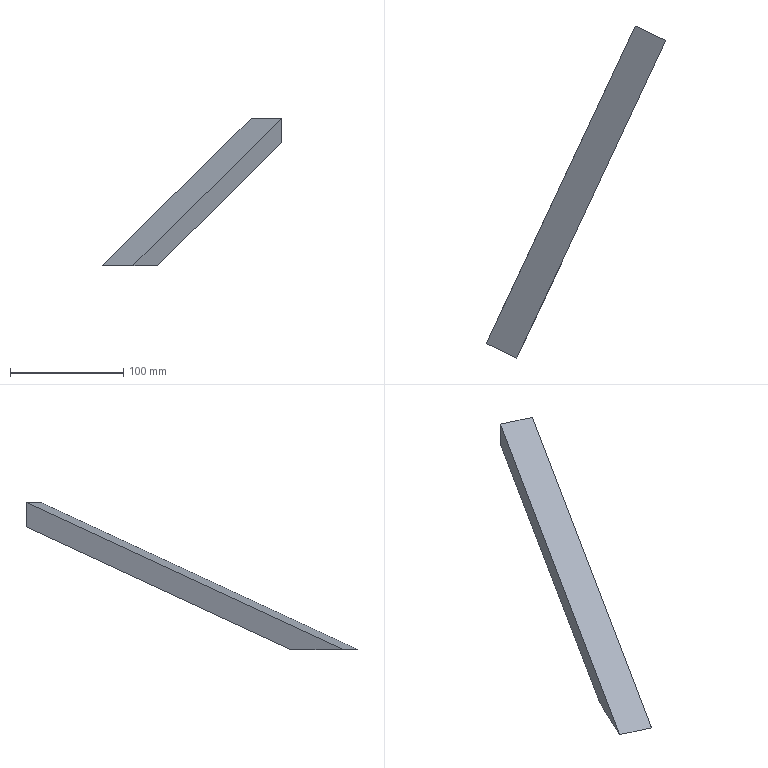Part | STEP file | Boss-Extrude 36 | 1 solid | 6 faces | box 158.76 x 293.326 x 130.156 mm | volume 184876 mm3 | plane 6
STEP:
#1=CARTESIAN_POINT('',(-1003.706,-516.863,2786.));
#2=VERTEX_POINT('',#1);
#3=CARTESIAN_POINT('',(-894.04,-283.039,2894.464));
#4=VERTEX_POINT('',#3);
#5=CARTESIAN_POINT('',(-894.04,-283.039,2894.464));
#6=DIRECTION('',(0.3915,0.8347,0.3872));
#7=VECTOR('',#6,1000.);
#8=LINE('',#5,#7);
#9=EDGE_CURVE('',#2,#4,#8,.T.);
#10=ORIENTED_EDGE('',*,*,#9,.F.);
#11=CARTESIAN_POINT('',(-1030.867,-504.124,2786.));
#12=VERTEX_POINT('',#11);
#13=CARTESIAN_POINT('',(-1030.867,-504.124,2786.));
#14=DIRECTION('',(0.9054,-0.4246,0.));
#15=VECTOR('',#14,1000.);
#16=LINE('',#13,#15);
#17=EDGE_CURVE('',#12,#2,#16,.T.);
#18=ORIENTED_EDGE('',*,*,#17,.F.);
#19=CARTESIAN_POINT('',(-921.201,-270.3,2894.464));
#20=VERTEX_POINT('',#19);
#21=CARTESIAN_POINT('',(-921.201,-270.3,2894.464));
#22=DIRECTION('',(0.3915,0.8347,0.3872));
#23=VECTOR('',#22,1000.);
#24=LINE('',#21,#23);
#25=EDGE_CURVE('',#12,#20,#24,.T.);
#26=ORIENTED_EDGE('',*,*,#25,.T.);
#27=CARTESIAN_POINT('',(-921.201,-270.3,2894.464));
#28=DIRECTION('',(0.9054,-0.4246,0.));
#29=VECTOR('',#28,1000.);
#30=LINE('',#27,#29);
#31=EDGE_CURVE('',#20,#4,#30,.T.);
#32=ORIENTED_EDGE('',*,*,#31,.T.);
#33=EDGE_LOOP('',(#10,#18,#26,#32));
#34=FACE_OUTER_BOUND('',#33,.T.);
#35=CARTESIAN_POINT('',(-921.201,-270.3,2894.464));
#36=DIRECTION('',(0.1644,0.3506,-0.922));
#37=DIRECTION('',(0.,-0.9347,-0.3554));
#38=AXIS2_PLACEMENT_3D('',#35,#36,#37);
#39=PLANE('',#38);
#40=ADVANCED_FACE('',(#34),#39,.T.);
#41=CARTESIAN_POINT('',(-1025.638,-563.627,2786.));
#42=VERTEX_POINT('',#41);
#43=CARTESIAN_POINT('',(-1003.706,-516.863,2786.));
#44=DIRECTION('',(0.4246,0.9054,0.));
#45=VECTOR('',#44,1000.);
#46=LINE('',#43,#45);
#47=EDGE_CURVE('',#42,#2,#46,.T.);
#48=ORIENTED_EDGE('',*,*,#47,.F.);
#49=CARTESIAN_POINT('',(-1052.799,-550.888,2786.));
#50=VERTEX_POINT('',#49);
#51=CARTESIAN_POINT('',(-1052.799,-550.888,2786.));
#52=DIRECTION('',(0.9054,-0.4246,0.));
#53=VECTOR('',#52,1000.);
#54=LINE('',#51,#53);
#55=EDGE_CURVE('',#50,#42,#54,.T.);
#56=ORIENTED_EDGE('',*,*,#55,.F.);
#57=CARTESIAN_POINT('',(-1030.867,-504.124,2786.));
#58=DIRECTION('',(0.4246,0.9054,0.));
#59=VECTOR('',#58,1000.);
#60=LINE('',#57,#59);
#61=EDGE_CURVE('',#50,#12,#60,.T.);
#62=ORIENTED_EDGE('',*,*,#61,.T.);
#63=ORIENTED_EDGE('',*,*,#17,.T.);
#64=EDGE_LOOP('',(#48,#56,#62,#63));
#65=FACE_OUTER_BOUND('',#64,.T.);
#66=CARTESIAN_POINT('',(-1030.867,-504.124,2786.));
#67=DIRECTION('',(0.,0.,-1.));
#68=DIRECTION('',(0.,-1.,0.));
#69=AXIS2_PLACEMENT_3D('',#66,#67,#68);
#70=PLANE('',#69);
#71=ADVANCED_FACE('',(#65),#70,.T.);
#72=CARTESIAN_POINT('',(-894.04,-283.039,2916.156));
#73=VERTEX_POINT('',#72);
#74=CARTESIAN_POINT('',(-1025.638,-563.627,2786.));
#75=DIRECTION('',(-0.3915,-0.8347,-0.3872));
#76=VECTOR('',#75,1000.);
#77=LINE('',#74,#76);
#78=EDGE_CURVE('',#73,#42,#77,.T.);
#79=ORIENTED_EDGE('',*,*,#78,.F.);
#80=CARTESIAN_POINT('',(-921.201,-270.3,2916.156));
#81=VERTEX_POINT('',#80);
#82=CARTESIAN_POINT('',(-921.201,-270.3,2916.156));
#83=DIRECTION('',(0.9054,-0.4246,0.));
#84=VECTOR('',#83,1000.);
#85=LINE('',#82,#84);
#86=EDGE_CURVE('',#81,#73,#85,.T.);
#87=ORIENTED_EDGE('',*,*,#86,.F.);
#88=CARTESIAN_POINT('',(-932.278,-293.919,2905.2));
#89=DIRECTION('',(-0.3915,-0.8347,-0.3872));
#90=VECTOR('',#89,1000.);
#91=LINE('',#88,#90);
#92=EDGE_CURVE('',#81,#50,#91,.T.);
#93=ORIENTED_EDGE('',*,*,#92,.T.);
#94=ORIENTED_EDGE('',*,*,#55,.T.);
#95=EDGE_LOOP('',(#79,#87,#93,#94));
#96=FACE_OUTER_BOUND('',#95,.T.);
#97=CARTESIAN_POINT('',(-1052.799,-550.888,2786.));
#98=DIRECTION('',(-0.1644,-0.3506,0.922));
#99=DIRECTION('',(0.,0.9347,0.3554));
#100=AXIS2_PLACEMENT_3D('',#97,#98,#99);
#101=PLANE('',#100);
#102=ADVANCED_FACE('',(#96),#101,.T.);
#103=CARTESIAN_POINT('',(-894.04,-283.039,2916.156));
#104=DIRECTION('',(0.,0.,1.));
#105=VECTOR('',#104,1000.);
#106=LINE('',#103,#105);
#107=EDGE_CURVE('',#4,#73,#106,.T.);
#108=ORIENTED_EDGE('',*,*,#107,.F.);
#109=ORIENTED_EDGE('',*,*,#31,.F.);
#110=CARTESIAN_POINT('',(-921.201,-270.3,2916.156));
#111=DIRECTION('',(0.,0.,1.));
#112=VECTOR('',#111,1000.);
#113=LINE('',#110,#112);
#114=EDGE_CURVE('',#20,#81,#113,.T.);
#115=ORIENTED_EDGE('',*,*,#114,.T.);
#116=ORIENTED_EDGE('',*,*,#86,.T.);
#117=EDGE_LOOP('',(#108,#109,#115,#116));
#118=FACE_OUTER_BOUND('',#117,.T.);
#119=CARTESIAN_POINT('',(-921.201,-270.3,2916.156));
#120=DIRECTION('',(0.4246,0.9054,0.));
#121=DIRECTION('',(0.9054,-0.4246,0.));
#122=AXIS2_PLACEMENT_3D('',#119,#120,#121);
#123=PLANE('',#122);
#124=ADVANCED_FACE('',(#118),#123,.T.);
#125=ORIENTED_EDGE('',*,*,#25,.F.);
#126=ORIENTED_EDGE('',*,*,#61,.F.);
#127=ORIENTED_EDGE('',*,*,#92,.F.);
#128=ORIENTED_EDGE('',*,*,#114,.F.);
#129=EDGE_LOOP('',(#125,#126,#127,#128));
#130=FACE_OUTER_BOUND('',#129,.T.);
#131=CARTESIAN_POINT('',(-1141.698,-740.433,2776.));
#132=DIRECTION('',(0.9054,-0.4246,0.));
#133=DIRECTION('',(-0.4246,-0.9054,0.));
#134=AXIS2_PLACEMENT_3D('',#131,#132,#133);
#135=PLANE('',#134);
#136=ADVANCED_FACE('',(#130),#135,.F.);
#137=ORIENTED_EDGE('',*,*,#9,.T.);
#138=ORIENTED_EDGE('',*,*,#107,.T.);
#139=ORIENTED_EDGE('',*,*,#78,.T.);
#140=ORIENTED_EDGE('',*,*,#47,.T.);
#141=EDGE_LOOP('',(#137,#138,#139,#140));
#142=FACE_OUTER_BOUND('',#141,.T.);
#143=CARTESIAN_POINT('',(-1114.537,-753.172,2776.));
#144=DIRECTION('',(0.9054,-0.4246,0.));
#145=DIRECTION('',(-0.4246,-0.9054,0.));
#146=AXIS2_PLACEMENT_3D('',#143,#144,#145);
#147=PLANE('',#146);
#148=ADVANCED_FACE('',(#142),#147,.T.);
#149=CLOSED_SHELL('',(#40,#71,#102,#124,#136,#148));
#150=MANIFOLD_SOLID_BREP('',#149);
#151=CARTESIAN_POINT('',(0.,0.,0.));
#152=DIRECTION('',(0.,0.,1.));
#153=DIRECTION('',(1.,0.,0.));
#154=AXIS2_PLACEMENT_3D('',#151,#152,#153);
#155=(LENGTH_UNIT()NAMED_UNIT(*)SI_UNIT(.MILLI.,.METRE.));
#156=UNCERTAINTY_MEASURE_WITH_UNIT(LENGTH_MEASURE(0.00001),#155,'','');
#157=(NAMED_UNIT(*)PLANE_ANGLE_UNIT()SI_UNIT($,.RADIAN.));
#158=(NAMED_UNIT(*)SI_UNIT($,.STERADIAN.)SOLID_ANGLE_UNIT());
#159=(GEOMETRIC_REPRESENTATION_CONTEXT(3)GLOBAL_UNCERTAINTY_ASSIGNED_CONTEXT((#156))GLOBAL_UNIT_ASSIGNED_CONTEXT((#155,#157,#158))REPRESENTATION_CONTEXT('',''));
#160=ADVANCED_BREP_SHAPE_REPRESENTATION('',(#150,#154),#159);